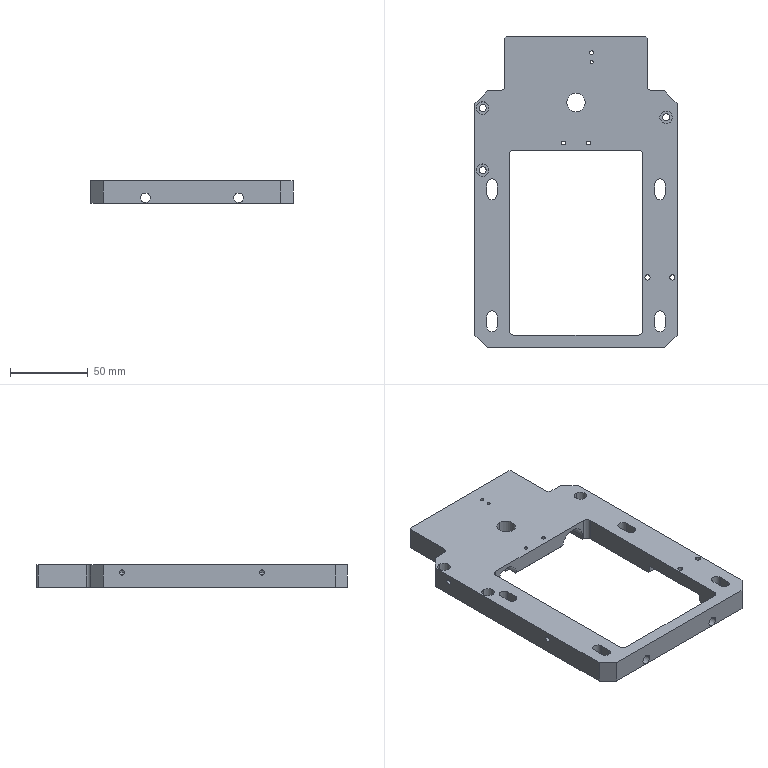NC program | NX | posted with a generic post | part box 130 x 200 x 14.5 mm
Whole program:
N10 G17 G21 G94 G90
(HOLE_MILLING_COPY , TOOL : D6)
N12 T06 M6
N14 G54
N16 G17 G0 G90 X-60. Y54. B0. C0. S5500 M3
N18 G43 Z30. H6
N20 Z0.5
N22 G94 G3 X-59.5 Y53.5 R0.5 F1500.
N24 X-59. Y54. R0.5
N26 X-59. Y54. Z0.4 I-1. J0.
N28 X-59. Y54. Z0.3 I-1. J0.
N30 X-59. Y54. Z0.2 I-1. J0.
N32 X-59. Y54. Z0.1 I-1. J0.
N34 X-59. Y54. Z0. I-1. J0.
N36 X-59. Y54. Z-0.1 I-1. J0.
N38 X-59. Y54. Z-0.2 I-1. J0.
N40 X-59. Y54. Z-0.3 I-1. J0.
N42 X-59. Y54. Z-0.4 I-1. J0.
N44 X-59. Y54. Z-0.5 I-1. J0.
N46 X-59. Y54. Z-0.6 I-1. J0.
N48 X-59. Y54. Z-0.7 I-1. J0.
N50 X-59. Y54. Z-0.8 I-1. J0.
N52 X-59. Y54. Z-0.9 I-1. J0.
N54 X-59. Y54. Z-1. I-1. J0.
N56 X-59. Y54. Z-1.1 I-1. J0.
N58 X-59. Y54. Z-1.2 I-1. J0.
N60 X-59. Y54. Z-1.3 I-1. J0.
N62 X-59. Y54. Z-1.4 I-1. J0.
N64 X-59. Y54. Z-1.5 I-1. J0.
N66 X-59. Y54. Z-1.6 I-1. J0.
N68 X-59. Y54. Z-1.7 I-1. J0.
N70 X-59. Y54. Z-1.8 I-1. J0.
N72 X-59. Y54. Z-1.9 I-1. J0.
N74 X-59. Y54. Z-2. I-1. J0.
N76 X-59. Y54. Z-2.1 I-1. J0.
N78 X-59. Y54. Z-2.2 I-1. J0.
N80 X-59. Y54. Z-2.3 I-1. J0.
N82 X-59. Y54. Z-2.4 I-1. J0.
N84 X-59. Y54. Z-2.5 I-1. J0.
N86 X-59. Y54. Z-2.6 I-1. J0.
N88 X-59. Y54. Z-2.7 I-1. J0.
N90 X-59. Y54. Z-2.8 I-1. J0.
N92 X-59. Y54. Z-2.9 I-1. J0.
N94 X-59. Y54. Z-3. I-1. J0.
N96 X-59. Y54. Z-3.1 I-1. J0.
N98 X-59. Y54. Z-3.2 I-1. J0.
N100 X-59. Y54. Z-3.3 I-1. J0.
N102 X-59. Y54. Z-3.4 I-1. J0.
N104 X-59. Y54. Z-3.5 I-1. J0.
N106 X-59. Y54. Z-3.6 I-1. J0.
N108 X-59. Y54. Z-3.7 I-1. J0.
N110 X-59. Y54. Z-3.8 I-1. J0.
N112 X-59. Y54. Z-3.9 I-1. J0.
N114 X-59. Y54. Z-4. I-1. J0.
N116 X-59. Y54. Z-4.1 I-1. J0.
N118 X-59. Y54. Z-4.2 I-1. J0.
N120 X-59. Y54. Z-4.3 I-1. J0.
N122 X-59. Y54. Z-4.4 I-1. J0.
N124 X-59. Y54. Z-4.5 I-1. J0.
N126 X-59. Y54. Z-4.6 I-1. J0.
N128 X-59. Y54. Z-4.7 I-1. J0.
N130 X-59. Y54. Z-4.8 I-1. J0.
N132 X-59. Y54. Z-4.9 I-1. J0.
N134 X-59. Y54. Z-5. I-1. J0.
N136 X-59. Y54. Z-5.1 I-1. J0.
N138 X-59. Y54. Z-5.2 I-1. J0.
N140 X-59. Y54. Z-5.3 I-1. J0.
N142 X-59. Y54. Z-5.4 I-1. J0.
N144 X-59. Y54. Z-5.5 I-1. J0.
N146 X-59. Y54. Z-5.6 I-1. J0.
N148 X-59. Y54. Z-5.7 I-1. J0.
N150 X-59. Y54. Z-5.8 I-1. J0.
N152 X-59. Y54. Z-5.9 I-1. J0.
N154 X-59. Y54. Z-6. I-1. J0.
N156 X-59. Y54. Z-6.1 I-1. J0.
N158 X-59. Y54. Z-6.2 I-1. J0.
N160 X-59. Y54. Z-6.3 I-1. J0.
N162 X-59. Y54. Z-6.4 I-1. J0.
N164 X-59. Y54. Z-6.5 I-1. J0.
N166 X-59. Y54. Z-6.6 I-1. J0.
N168 X-60. Y55. R1.
N170 X-59. Y54. R-1.
N172 X-59.5 Y54.5 R0.5
N174 X-60. Y54. R0.5
N176 G0 Z30.
N178 Y14.
N180 Z0.5
N182 G3 X-59.5 Y13.5 R0.5
N184 X-59. Y14. R0.5
N186 X-59. Y14. Z0.4 I-1. J0.
N188 X-59. Y14. Z0.3 I-1. J0.
N190 X-59. Y14. Z0.2 I-1. J0.
N192 X-59. Y14. Z0.1 I-1. J0.
N194 X-59. Y14. Z0. I-1. J0.
N196 X-59. Y14. Z-0.1 I-1. J0.
N198 X-59. Y14. Z-0.2 I-1. J0.
N200 X-59. Y14. Z-0.3 I-1. J0.
N202 X-59. Y14. Z-0.4 I-1. J0.
N204 X-59. Y14. Z-0.5 I-1. J0.
N206 X-59. Y14. Z-0.6 I-1. J0.
N208 X-59. Y14. Z-0.7 I-1. J0.
N210 X-59. Y14. Z-0.8 I-1. J0.
N212 X-59. Y14. Z-0.9 I-1. J0.
N214 X-59. Y14. Z-1. I-1. J0.
N216 X-59. Y14. Z-1.1 I-1. J0.
N218 X-59. Y14. Z-1.2 I-1. J0.
N220 X-59. Y14. Z-1.3 I-1. J0.
N222 X-59. Y14. Z-1.4 I-1. J0.
N224 X-59. Y14. Z-1.5 I-1. J0.
N226 X-59. Y14. Z-1.6 I-1. J0.
N228 X-59. Y14. Z-1.7 I-1. J0.
N230 X-59. Y14. Z-1.8 I-1. J0.
N232 X-59. Y14. Z-1.9 I-1. J0.
N234 X-59. Y14. Z-2. I-1. J0.
N236 X-59. Y14. Z-2.1 I-1. J0.
N238 X-59. Y14. Z-2.2 I-1. J0.
N240 X-59. Y14. Z-2.3 I-1. J0.
N242 X-59. Y14. Z-2.4 I-1. J0.
N244 X-59. Y14. Z-2.5 I-1. J0.
N246 X-59. Y14. Z-2.6 I-1. J0.
N248 X-59. Y14. Z-2.7 I-1. J0.
N250 X-59. Y14. Z-2.8 I-1. J0.
N252 X-59. Y14. Z-2.9 I-1. J0.
N254 X-59. Y14. Z-3. I-1. J0.
N256 X-59. Y14. Z-3.1 I-1. J0.
N258 X-59. Y14. Z-3.2 I-1. J0.
N260 X-59. Y14. Z-3.3 I-1. J0.
N262 X-59. Y14. Z-3.4 I-1. J0.
N264 X-59. Y14. Z-3.5 I-1. J0.
N266 X-59. Y14. Z-3.6 I-1. J0.
N268 X-59. Y14. Z-3.7 I-1. J0.
N270 X-59. Y14. Z-3.8 I-1. J0.
N272 X-59. Y14. Z-3.9 I-1. J0.
N274 X-59. Y14. Z-4. I-1. J0.
N276 X-59. Y14. Z-4.1 I-1. J0.
N278 X-59. Y14. Z-4.2 I-1. J0.
N280 X-59. Y14. Z-4.3 I-1. J0.
N282 X-59. Y14. Z-4.4 I-1. J0.
N284 X-59. Y14. Z-4.5 I-1. J0.
N286 X-59. Y14. Z-4.6 I-1. J0.
N288 X-59. Y14. Z-4.7 I-1. J0.
N290 X-59. Y14. Z-4.8 I-1. J0.
N292 X-59. Y14. Z-4.9 I-1. J0.
N294 X-59. Y14. Z-5. I-1. J0.
N296 X-59. Y14. Z-5.1 I-1. J0.
N298 X-59. Y14. Z-5.2 I-1. J0.
N300 X-59. Y14. Z-5.3 I-1. J0.
N302 X-59. Y14. Z-5.4 I-1. J0.
N304 X-59. Y14. Z-5.5 I-1. J0.
N306 X-59. Y14. Z-5.6 I-1. J0.
N308 X-59. Y14. Z-5.7 I-1. J0.
N310 X-59. Y14. Z-5.8 I-1. J0.
N312 X-59. Y14. Z-5.9 I-1. J0.
N314 X-59. Y14. Z-6. I-1. J0.
N316 X-59. Y14. Z-6.1 I-1. J0.
N318 X-59. Y14. Z-6.2 I-1. J0.
N320 X-59. Y14. Z-6.3 I-1. J0.
N322 X-59. Y14. Z-6.4 I-1. J0.
N324 X-59. Y14. Z-6.5 I-1. J0.
N326 X-59. Y14. Z-6.6 I-1. J0.
N328 X-60. Y15. R1.
N330 X-59. Y14. R-1.
N332 X-59.5 Y14.5 R0.5
N334 X-60. Y14. R0.5
N336 G0 Z30.
N338 X58. Y48.
N340 Z0.5
N342 G3 X58.5 Y47.5 R0.5
N344 X59. Y48. R0.5
N346 X59. Y48. Z0.4 I-1. J0.
N348 X59. Y48. Z0.3 I-1. J0.
N350 X59. Y48. Z0.2 I-1. J0.
N352 X59. Y48. Z0.1 I-1. J0.
N354 X59. Y48. Z0. I-1. J0.
N356 X59. Y48. Z-0.1 I-1. J0.
N358 X59. Y48. Z-0.2 I-1. J0.
N360 X59. Y48. Z-0.3 I-1. J0.
N362 X59. Y48. Z-0.4 I-1. J0.
N364 X59. Y48. Z-0.5 I-1. J0.
N366 X59. Y48. Z-0.6 I-1. J0.
N368 X59. Y48. Z-0.7 I-1. J0.
N370 X59. Y48. Z-0.8 I-1. J0.
N372 X59. Y48. Z-0.9 I-1. J0.
N374 X59. Y48. Z-1. I-1. J0.
N376 X59. Y48. Z-1.1 I-1. J0.
N378 X59. Y48. Z-1.2 I-1. J0.
N380 X59. Y48. Z-1.3 I-1. J0.
N382 X59. Y48. Z-1.4 I-1. J0.
N384 X59. Y48. Z-1.5 I-1. J0.
N386 X59. Y48. Z-1.6 I-1. J0.
N388 X59. Y48. Z-1.7 I-1. J0.
N390 X59. Y48. Z-1.8 I-1. J0.
N392 X59. Y48. Z-1.9 I-1. J0.
N394 X59. Y48. Z-2. I-1. J0.
N396 X59. Y48. Z-2.1 I-1. J0.
N398 X59. Y48. Z-2.2 I-1. J0.
N400 X59. Y48. Z-2.3 I-1. J0.
N402 X59. Y48. Z-2.4 I-1. J0.
N404 X59. Y48. Z-2.5 I-1. J0.
N406 X59. Y48. Z-2.6 I-1. J0.
N408 X59. Y48. Z-2.7 I-1. J0.
N410 X59. Y48. Z-2.8 I-1. J0.
N412 X59. Y48. Z-2.9 I-1. J0.
N414 X59. Y48. Z-3. I-1. J0.
N416 X59. Y48. Z-3.1 I-1. J0.
N418 X59. Y48. Z-3.2 I-1. J0.
N420 X59. Y48. Z-3.3 I-1. J0.
N422 X59. Y48. Z-3.4 I-1. J0.
N424 X59. Y48. Z-3.5 I-1. J0.
N426 X59. Y48. Z-3.6 I-1. J0.
N428 X59. Y48. Z-3.7 I-1. J0.
N430 X59. Y48. Z-3.8 I-1. J0.
N432 X59. Y48. Z-3.9 I-1. J0.
N434 X59. Y48. Z-4. I-1. J0.
N436 X59. Y48. Z-4.1 I-1. J0.
N438 X59. Y48. Z-4.2 I-1. J0.
N440 X59. Y48. Z-4.3 I-1. J0.
N442 X59. Y48. Z-4.4 I-1. J0.
N444 X59. Y48. Z-4.5 I-1. J0.
N446 X59. Y48. Z-4.6 I-1. J0.
N448 X59. Y48. Z-4.7 I-1. J0.
N450 X59. Y48. Z-4.8 I-1. J0.
N452 X59. Y48. Z-4.9 I-1. J0.
N454 X59. Y48. Z-5. I-1. J0.
N456 X59. Y48. Z-5.1 I-1. J0.
N458 X59. Y48. Z-5.2 I-1. J0.
N460 X59. Y48. Z-5.3 I-1. J0.
N462 X59. Y48. Z-5.4 I-1. J0.
N464 X59. Y48. Z-5.5 I-1. J0.
N466 X59. Y48. Z-5.6 I-1. J0.
N468 X59. Y48. Z-5.7 I-1. J0.
N470 X59. Y48. Z-5.8 I-1. J0.
N472 X59. Y48. Z-5.9 I-1. J0.
N474 X59. Y48. Z-6. I-1. J0.
N476 X59. Y48. Z-6.1 I-1. J0.
N478 X59. Y48. Z-6.2 I-1. J0.
N480 X59. Y48. Z-6.3 I-1. J0.
N482 X59. Y48. Z-6.4 I-1. J0.
N484 X59. Y48. Z-6.5 I-1. J0.
N486 X59. Y48. Z-6.6 I-1. J0.
N488 X58. Y49. R1.
N490 X59. Y48. R-1.
N492 X58.5 Y48.5 R0.5
N494 X58. Y48. R0.5
N496 G0 Z30.
N498 M5
(PLANAR_MILL_COPY_1 , TOOL : D6A45)
N500 T01 M6
N502 G54
N504 G17 G0 G90 X-62.743 Y54.766 B0. C0. S7500 M3
N506 G43 Z30. H1
N508 Z1.
N510 G94 G1 Z-1. F1250.
N512 G3 X-63.1 Y54. R1.
N514 X-60. Y50.9 R3.1
N516 X-63.1 Y54. R-3.1
N518 X-62.743 Y53.234 R1.
N520 G1 Z1.
N522 G0 Z30.
N524 Y14.766
N526 Z1.
N528 G1 Z-1.
N530 G3 X-63.1 Y14. R1.
N532 X-60. Y10.9 R3.1
N534 X-63.1 Y14. R-3.1
N536 X-62.743 Y13.234 R1.
N538 G1 Z1.
N540 G0 Z30.
N542 X-55.993 Y2.516
N544 Z1.
N546 G1 Z-1.
N548 G3 X-56.35 Y1.75 R1.
N550 G1 Y-1.75
N552 G3 X-54. Y-4.1 R2.35
N554 X-51.65 Y-1.75 R2.35
N556 G1 Y5.25
N558 G3 X-54. Y7.6 R2.35
N560 X-56.35 Y5.25 R2.35
N562 G1 Y1.75
N564 G3 X-55.993 Y0.984 R1.
N566 G1 Z1.
N568 G0 Z30.
N570 X-66.257 Y-18.266
N572 Z1.
N574 G1 Z-1.
N576 G3 X-65.9 Y-17.5 R1.
N578 G1 Y57.
N580 G2 X-65.636 Y57.636 R0.9
N582 G1 X-57.636 Y65.636
N584 G2 X-57. Y65.9 R0.9
N586 G1 X-49.
N588 G3 X-46.9 Y68. R2.1
N590 G1 Y99.
N592 G2 X-46.636 Y99.636 R0.9
N594 G1 X-45.636 Y100.636
N596 G2 X-45. Y100.9 R0.9
N598 G1 X45.
N600 G2 X45.636 Y100.636 R0.9
N602 G1 X46.636 Y99.636
N604 G2 X46.9 Y99. R0.9
N606 G1 Y68.
N608 G3 X49. Y65.9 R2.1
N610 G1 X57.
N612 G2 X57.636 Y65.636 R0.9
N614 G1 X65.636 Y57.636
N616 G2 X65.9 Y57. R0.9
N618 G1 Y-92.
N620 G2 X65.636 Y-92.636 R0.9
N622 G1 X57.636 Y-100.636
N624 G2 X57. Y-100.9 R0.9
N626 G1 X-57.
N628 G2 X-57.636 Y-100.636 R0.9
N630 G1 X-65.636 Y-92.636
N632 G2 X-65.9 Y-92. R0.9
N634 G1 Y-17.5
N636 G3 X-66.257 Y-16.734 R1.
N638 G1 Z1.
N640 G0 Z30.
N642 X7.93 Y31.547
N644 Z1.
N646 G1 Z-1.
N648 G3 X8.35 Y31.5 R0.5
N650 X8. Y31.85 R0.35
N652 X8.35 Y31.5 R-0.35
N654 X7.93 Y31.453 R0.5
N656 G1 Z1.
N658 G0 Z30.
N660 X-7.93
N662 Z1.
N664 G1 Z-1.
N666 G3 X-8.35 Y31.5 R0.5
N668 X-8. Y31.15 R0.35
N670 X-8.35 Y31.5 R-0.35
N672 X-7.93 Y31.547 R0.5
N674 G1 Z1.
N676 G0 Z30.
N678 X0.766 Y62.243
N680 Z1.
N682 G1 Z-1.
N684 G3 X0. Y62.6 R1.
N686 X-5.1 Y57.5 R5.1
N688 X0. Y62.6 R-5.1
N690 X-0.766 Y62.243 R1.
N692 G1 Z1.
N694 G0 Z30.
N696 X9.953 Y89.43
N698 Z1.
N700 G1 Z-1.
N702 G3 X10. Y89.85 R0.5
N704 X9.65 Y89.5 R0.35
N706 X10. Y89.85 R-0.35
N708 X10.047 Y89.43 R0.5
N710 G1 Z1.
N712 G0 Z30.
N714 X9.9 Y83.551
N716 Z1.
N718 G1 Y83.417 Z0.964
N720 X9.917 Y83.4 Z0.958
N722 X10.1 Y83.417 Z0.907
N724 X10.083 Y83.6 Z0.856
N726 X9.9 Y83.583 Z0.805
N728 X9.917 Y83.4 Z0.754
N730 X10.1 Y83.417 Z0.703
N732 X10.083 Y83.6 Z0.652
N734 X9.9 Y83.583 Z0.601
N736 X9.917 Y83.4 Z0.55
N738 X10.1 Y83.417 Z0.499
N740 X10.083 Y83.6 Z0.448
N742 X9.9 Y83.583 Z0.397
N744 X9.917 Y83.4 Z0.346
N746 X10.1 Y83.417 Z0.296
N748 X10.083 Y83.6 Z0.245
N750 X9.9 Y83.583 Z0.194
N752 X9.917 Y83.4 Z0.143
N754 X10.1 Y83.417 Z0.092
N756 X10.083 Y83.6 Z0.041
N758 X9.9 Y83.583 Z-0.01
N760 X9.917 Y83.4 Z-0.061
N762 X10.1 Y83.417 Z-0.112
N764 X10.083 Y83.6 Z-0.163
N766 X9.9 Y83.583 Z-0.214
N768 X9.917 Y83.4 Z-0.265
N770 X10.1 Y83.417 Z-0.316
N772 X10.083 Y83.6 Z-0.367
N774 X9.9 Y83.583 Z-0.417
N776 X9.917 Y83.4 Z-0.468
N778 X10.1 Y83.417 Z-0.519
N780 X10.083 Y83.6 Z-0.57
N782 X9.9 Y83.583 Z-0.621
N784 X9.917 Y83.4 Z-0.672
N786 X10.1 Y83.417 Z-0.723
N788 X10.083 Y83.6 Z-0.774
N790 X9.9 Y83.583 Z-0.825
N792 X9.917 Y83.4 Z-0.876
N794 X10.1 Y83.417 Z-0.927
N796 X10.083 Y83.6 Z-0.978
N798 X10. Z-1.
N800 G3 X9.9 Y83.5 R0.1
N802 X10. Y83.6 R-0.1
N804 G1 Z1.
N806 G0 Z30.
N808 X60.743 Y47.234
N810 Z1.
N812 G1 Z-1.
N814 G3 X61.1 Y48. R1.
N816 X58. Y51.1 R3.1
N818 X61.1 Y48. R-3.1
N820 X60.743 Y48.766 R1.
N822 G1 Z1.
N824 G0 Z30.
N826 X55.993 Y0.984
N828 Z1.
N830 G1 Z-1.
N832 G3 X56.35 Y1.75 R1.
N834 G1 Y5.25
N836 G3 X54. Y7.6 R2.35
N838 X51.65 Y5.25 R2.35
N840 G1 Y-1.75
N842 G3 X54. Y-4.1 R2.35
N844 X56.35 Y-1.75 R2.35
N846 G1 Y1.75
N848 G3 X55.993 Y2.516 R1.
N850 G1 Z1.
N852 G0 Z30.
N854 X62.571 Y-55.383
N856 Z1.
N858 G1 Z-1.
N860 G3 X62.75 Y-55. R0.5
N862 X62. Y-54.25 R0.75
N864 X62.75 Y-55. R-0.75
N866 X62.571 Y-54.617 R0.5
N868 G1 Z1.
N870 G0 Z30.
N872 X55.993 Y-84.016
N874 Z1.
N876 G1 Z-1.
N878 G3 X56.35 Y-83.25 R1.
N880 G1 Y-79.75
N882 G3 X54. Y-77.4 R2.35
N884 X51.65 Y-79.75 R2.35
N886 G1 Y-86.75
N888 G3 X54. Y-89.1 R2.35
N890 X56.35 Y-86.75 R2.35
N892 G1 Y-83.25
N894 G3 X55.993 Y-82.484 R1.
N896 G1 Z1.
N898 G0 Z30.
N900 X46.571 Y-55.383
N902 Z1.
N904 G1 Z-1.
N906 G3 X46.75 Y-55. R0.5
N908 X46. Y-54.25 R0.75
N910 X46.75 Y-55. R-0.75
N912 X46.571 Y-54.617 R0.5
N914 G1 Z1.
N916 G0 Z30.
N918 X41.743 Y-33.266
N920 Z1.
N922 G1 Z-1.
N924 G3 X42.1 Y-32.5 R1.
N926 G1 Y24.
N928 G3 X40. Y26.1 R2.1
N930 G1 X-40.
N932 G3 X-42.1 Y24. R2.1
N934 G1 Y-89.
N936 G3 X-40. Y-91.1 R2.1
N938 G1 X40.
N940 G3 X42.1 Y-89. R2.1
N942 G1 Y-32.5
N944 G3 X41.743 Y-31.734 R1.
N946 G1 Z1.
N948 G0 Z30.
N950 X-55.993 Y-82.484
N952 Z1.
N954 G1 Z-1.
N956 G3 X-56.35 Y-83.25 R1.
N958 G1 Y-86.75
N960 G3 X-54. Y-89.1 R2.35
N962 X-51.65 Y-86.75 R2.35
N964 G1 Y-79.75
N966 G3 X-54. Y-77.4 R2.35
N968 X-56.35 Y-79.75 R2.35
N970 G1 Y-83.25
N972 G3 X-55.993 Y-84.016 R1.
N974 G1 Z1.
N976 G0 Z30.
N978 M5
N980 M2